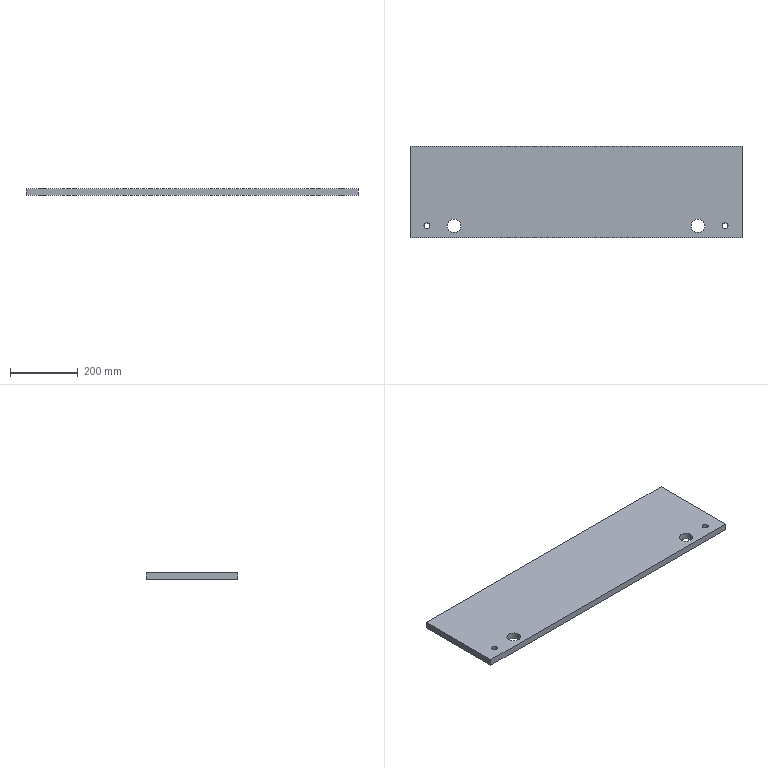Part | STEP file | Base Plate | 1 solid | 14 faces | box 980 x 270 x 20 mm | volume 5232113 mm3 | cylinder 8 | plane 6 | commonest cylinder face diameters 17.5 x4 40 x4
STEP:
#1=CARTESIAN_POINT('',(0.,0.,0.));
#2=DIRECTION('',(0.,0.,1.));
#3=DIRECTION('',(1.,0.,0.));
#4=AXIS2_PLACEMENT_3D('',#1,#2,#3);
#5=CARTESIAN_POINT('',(-340.,-100.,0.));
#6=VERTEX_POINT('',#5);
#7=CARTESIAN_POINT('',(-340.,-100.,20.));
#8=VERTEX_POINT('',#7);
#9=CARTESIAN_POINT('',(-340.,-100.,20.));
#10=DIRECTION('',(0.,0.,1.));
#11=VECTOR('',#10,1.);
#12=LINE('',#9,#11);
#13=CARTESIAN_POINT('',(-360.,-100.,20.));
#14=DIRECTION('',(0.,0.,1.));
#15=DIRECTION('',(1.,0.,0.));
#16=AXIS2_PLACEMENT_3D('',#13,#14,#15);
#17=CYLINDRICAL_SURFACE('',#16,20.);
#18=CARTESIAN_POINT('',(6.283,0.));
#19=DIRECTION('',(0.,1.));
#20=VECTOR('',#19,1.);
#21=LINE('',#18,#20);
#22=(GEOMETRIC_REPRESENTATION_CONTEXT(2)PARAMETRIC_REPRESENTATION_CONTEXT()REPRESENTATION_CONTEXT('',''));
#23=DEFINITIONAL_REPRESENTATION('',(#21),#22);
#24=PCURVE('',#17,#23);
#25=CARTESIAN_POINT('',(-360.,-100.,20.));
#26=DIRECTION('',(0.,0.,1.));
#27=DIRECTION('',(1.,0.,0.));
#28=AXIS2_PLACEMENT_3D('',#25,#26,#27);
#29=CYLINDRICAL_SURFACE('',#28,20.);
#30=CARTESIAN_POINT('',(0.,0.));
#31=DIRECTION('',(0.,1.));
#32=VECTOR('',#31,1.);
#33=LINE('',#30,#32);
#34=(GEOMETRIC_REPRESENTATION_CONTEXT(2)PARAMETRIC_REPRESENTATION_CONTEXT()REPRESENTATION_CONTEXT('',''));
#35=DEFINITIONAL_REPRESENTATION('',(#33),#34);
#36=PCURVE('',#29,#35);
#37=SURFACE_CURVE('',#12,(#24,#36),.PCURVE_S1.);
#38=EDGE_CURVE('',#6,#8,#37,.T.);
#39=ORIENTED_EDGE('',*,*,#38,.T.);
#40=CARTESIAN_POINT('',(-380.,-100.,20.));
#41=VERTEX_POINT('',#40);
#42=CARTESIAN_POINT('',(-360.,-100.,20.));
#43=DIRECTION('',(0.,0.,1.));
#44=DIRECTION('',(1.,0.,0.));
#45=AXIS2_PLACEMENT_3D('',#42,#43,#44);
#46=CIRCLE('',#45,20.);
#47=CARTESIAN_POINT('',(0.,0.));
#48=DIRECTION('',(1.,0.));
#49=VECTOR('',#48,1.);
#50=LINE('',#47,#49);
#51=(GEOMETRIC_REPRESENTATION_CONTEXT(2)PARAMETRIC_REPRESENTATION_CONTEXT()REPRESENTATION_CONTEXT('',''));
#52=DEFINITIONAL_REPRESENTATION('',(#50),#51);
#53=PCURVE('',#17,#52);
#54=CARTESIAN_POINT('',(0.,0.,20.));
#55=DIRECTION('',(0.,0.,1.));
#56=DIRECTION('',(1.,0.,0.));
#57=AXIS2_PLACEMENT_3D('',#54,#55,#56);
#58=PLANE('',#57);
#59=CARTESIAN_POINT('',(-360.,-100.));
#60=DIRECTION('',(1.,0.));
#61=AXIS2_PLACEMENT_2D('',#59,#60);
#62=CIRCLE('',#61,20.);
#63=(GEOMETRIC_REPRESENTATION_CONTEXT(2)PARAMETRIC_REPRESENTATION_CONTEXT()REPRESENTATION_CONTEXT('',''));
#64=DEFINITIONAL_REPRESENTATION('',(#62),#63);
#65=PCURVE('',#58,#64);
#66=SURFACE_CURVE('',#46,(#53,#65),.PCURVE_S1.);
#67=EDGE_CURVE('',#41,#8,#66,.T.);
#68=ORIENTED_EDGE('',*,*,#67,.F.);
#69=CARTESIAN_POINT('',(-380.,-100.,0.));
#70=VERTEX_POINT('',#69);
#71=CARTESIAN_POINT('',(-380.,-100.,20.));
#72=DIRECTION('',(0.,0.,1.));
#73=VECTOR('',#72,1.);
#74=LINE('',#71,#73);
#75=CARTESIAN_POINT('',(3.142,0.));
#76=DIRECTION('',(0.,1.));
#77=VECTOR('',#76,1.);
#78=LINE('',#75,#77);
#79=(GEOMETRIC_REPRESENTATION_CONTEXT(2)PARAMETRIC_REPRESENTATION_CONTEXT()REPRESENTATION_CONTEXT('',''));
#80=DEFINITIONAL_REPRESENTATION('',(#78),#79);
#81=PCURVE('',#17,#80);
#82=CARTESIAN_POINT('',(3.142,0.));
#83=DIRECTION('',(0.,1.));
#84=VECTOR('',#83,1.);
#85=LINE('',#82,#84);
#86=(GEOMETRIC_REPRESENTATION_CONTEXT(2)PARAMETRIC_REPRESENTATION_CONTEXT()REPRESENTATION_CONTEXT('',''));
#87=DEFINITIONAL_REPRESENTATION('',(#85),#86);
#88=PCURVE('',#29,#87);
#89=SURFACE_CURVE('',#74,(#81,#88),.PCURVE_S1.);
#90=EDGE_CURVE('',#70,#41,#89,.T.);
#91=ORIENTED_EDGE('',*,*,#90,.F.);
#92=CARTESIAN_POINT('',(-360.,-100.,0.));
#93=DIRECTION('',(0.,0.,1.));
#94=DIRECTION('',(1.,0.,0.));
#95=AXIS2_PLACEMENT_3D('',#92,#93,#94);
#96=CIRCLE('',#95,20.);
#97=CARTESIAN_POINT('',(0.,-20.));
#98=DIRECTION('',(1.,0.));
#99=VECTOR('',#98,1.);
#100=LINE('',#97,#99);
#101=(GEOMETRIC_REPRESENTATION_CONTEXT(2)PARAMETRIC_REPRESENTATION_CONTEXT()REPRESENTATION_CONTEXT('',''));
#102=DEFINITIONAL_REPRESENTATION('',(#100),#101);
#103=PCURVE('',#17,#102);
#104=CARTESIAN_POINT('',(0.,0.,0.));
#105=DIRECTION('',(0.,0.,1.));
#106=DIRECTION('',(1.,0.,0.));
#107=AXIS2_PLACEMENT_3D('',#104,#105,#106);
#108=PLANE('',#107);
#109=CARTESIAN_POINT('',(-360.,-100.));
#110=DIRECTION('',(1.,0.));
#111=AXIS2_PLACEMENT_2D('',#109,#110);
#112=CIRCLE('',#111,20.);
#113=(GEOMETRIC_REPRESENTATION_CONTEXT(2)PARAMETRIC_REPRESENTATION_CONTEXT()REPRESENTATION_CONTEXT('',''));
#114=DEFINITIONAL_REPRESENTATION('',(#112),#113);
#115=PCURVE('',#108,#114);
#116=SURFACE_CURVE('',#96,(#103,#115),.PCURVE_S1.);
#117=EDGE_CURVE('',#70,#6,#116,.T.);
#118=ORIENTED_EDGE('',*,*,#117,.T.);
#119=EDGE_LOOP('',(#39,#68,#91,#118));
#120=FACE_BOUND('',#119,.F.);
#121=ADVANCED_FACE('',(#120),#17,.F.);
#122=CARTESIAN_POINT('',(380.,-100.,0.));
#123=VERTEX_POINT('',#122);
#124=CARTESIAN_POINT('',(380.,-100.,20.));
#125=VERTEX_POINT('',#124);
#126=CARTESIAN_POINT('',(380.,-100.,20.));
#127=DIRECTION('',(0.,0.,1.));
#128=VECTOR('',#127,1.);
#129=LINE('',#126,#128);
#130=CARTESIAN_POINT('',(360.,-100.,20.));
#131=DIRECTION('',(0.,0.,1.));
#132=DIRECTION('',(1.,0.,0.));
#133=AXIS2_PLACEMENT_3D('',#130,#131,#132);
#134=CYLINDRICAL_SURFACE('',#133,20.);
#135=CARTESIAN_POINT('',(6.283,0.));
#136=DIRECTION('',(0.,1.));
#137=VECTOR('',#136,1.);
#138=LINE('',#135,#137);
#139=(GEOMETRIC_REPRESENTATION_CONTEXT(2)PARAMETRIC_REPRESENTATION_CONTEXT()REPRESENTATION_CONTEXT('',''));
#140=DEFINITIONAL_REPRESENTATION('',(#138),#139);
#141=PCURVE('',#134,#140);
#142=CARTESIAN_POINT('',(360.,-100.,20.));
#143=DIRECTION('',(0.,0.,1.));
#144=DIRECTION('',(1.,0.,0.));
#145=AXIS2_PLACEMENT_3D('',#142,#143,#144);
#146=CYLINDRICAL_SURFACE('',#145,20.);
#147=CARTESIAN_POINT('',(0.,0.));
#148=DIRECTION('',(0.,1.));
#149=VECTOR('',#148,1.);
#150=LINE('',#147,#149);
#151=(GEOMETRIC_REPRESENTATION_CONTEXT(2)PARAMETRIC_REPRESENTATION_CONTEXT()REPRESENTATION_CONTEXT('',''));
#152=DEFINITIONAL_REPRESENTATION('',(#150),#151);
#153=PCURVE('',#146,#152);
#154=SURFACE_CURVE('',#129,(#141,#153),.PCURVE_S1.);
#155=EDGE_CURVE('',#123,#125,#154,.T.);
#156=ORIENTED_EDGE('',*,*,#155,.T.);
#157=CARTESIAN_POINT('',(340.,-100.,20.));
#158=VERTEX_POINT('',#157);
#159=CARTESIAN_POINT('',(360.,-100.,20.));
#160=DIRECTION('',(0.,0.,1.));
#161=DIRECTION('',(1.,0.,0.));
#162=AXIS2_PLACEMENT_3D('',#159,#160,#161);
#163=CIRCLE('',#162,20.);
#164=CARTESIAN_POINT('',(0.,0.));
#165=DIRECTION('',(1.,0.));
#166=VECTOR('',#165,1.);
#167=LINE('',#164,#166);
#168=(GEOMETRIC_REPRESENTATION_CONTEXT(2)PARAMETRIC_REPRESENTATION_CONTEXT()REPRESENTATION_CONTEXT('',''));
#169=DEFINITIONAL_REPRESENTATION('',(#167),#168);
#170=PCURVE('',#134,#169);
#171=CARTESIAN_POINT('',(360.,-100.));
#172=DIRECTION('',(1.,0.));
#173=AXIS2_PLACEMENT_2D('',#171,#172);
#174=CIRCLE('',#173,20.);
#175=(GEOMETRIC_REPRESENTATION_CONTEXT(2)PARAMETRIC_REPRESENTATION_CONTEXT()REPRESENTATION_CONTEXT('',''));
#176=DEFINITIONAL_REPRESENTATION('',(#174),#175);
#177=PCURVE('',#58,#176);
#178=SURFACE_CURVE('',#163,(#170,#177),.PCURVE_S1.);
#179=EDGE_CURVE('',#158,#125,#178,.T.);
#180=ORIENTED_EDGE('',*,*,#179,.F.);
#181=CARTESIAN_POINT('',(340.,-100.,0.));
#182=VERTEX_POINT('',#181);
#183=CARTESIAN_POINT('',(340.,-100.,20.));
#184=DIRECTION('',(0.,0.,1.));
#185=VECTOR('',#184,1.);
#186=LINE('',#183,#185);
#187=CARTESIAN_POINT('',(3.142,0.));
#188=DIRECTION('',(0.,1.));
#189=VECTOR('',#188,1.);
#190=LINE('',#187,#189);
#191=(GEOMETRIC_REPRESENTATION_CONTEXT(2)PARAMETRIC_REPRESENTATION_CONTEXT()REPRESENTATION_CONTEXT('',''));
#192=DEFINITIONAL_REPRESENTATION('',(#190),#191);
#193=PCURVE('',#134,#192);
#194=CARTESIAN_POINT('',(3.142,0.));
#195=DIRECTION('',(0.,1.));
#196=VECTOR('',#195,1.);
#197=LINE('',#194,#196);
#198=(GEOMETRIC_REPRESENTATION_CONTEXT(2)PARAMETRIC_REPRESENTATION_CONTEXT()REPRESENTATION_CONTEXT('',''));
#199=DEFINITIONAL_REPRESENTATION('',(#197),#198);
#200=PCURVE('',#146,#199);
#201=SURFACE_CURVE('',#186,(#193,#200),.PCURVE_S1.);
#202=EDGE_CURVE('',#182,#158,#201,.T.);
#203=ORIENTED_EDGE('',*,*,#202,.F.);
#204=CARTESIAN_POINT('',(360.,-100.,0.));
#205=DIRECTION('',(0.,0.,1.));
#206=DIRECTION('',(1.,0.,0.));
#207=AXIS2_PLACEMENT_3D('',#204,#205,#206);
#208=CIRCLE('',#207,20.);
#209=CARTESIAN_POINT('',(0.,-20.));
#210=DIRECTION('',(1.,0.));
#211=VECTOR('',#210,1.);
#212=LINE('',#209,#211);
#213=(GEOMETRIC_REPRESENTATION_CONTEXT(2)PARAMETRIC_REPRESENTATION_CONTEXT()REPRESENTATION_CONTEXT('',''));
#214=DEFINITIONAL_REPRESENTATION('',(#212),#213);
#215=PCURVE('',#134,#214);
#216=CARTESIAN_POINT('',(360.,-100.));
#217=DIRECTION('',(1.,0.));
#218=AXIS2_PLACEMENT_2D('',#216,#217);
#219=CIRCLE('',#218,20.);
#220=(GEOMETRIC_REPRESENTATION_CONTEXT(2)PARAMETRIC_REPRESENTATION_CONTEXT()REPRESENTATION_CONTEXT('',''));
#221=DEFINITIONAL_REPRESENTATION('',(#219),#220);
#222=PCURVE('',#108,#221);
#223=SURFACE_CURVE('',#208,(#215,#222),.PCURVE_S1.);
#224=EDGE_CURVE('',#182,#123,#223,.T.);
#225=ORIENTED_EDGE('',*,*,#224,.T.);
#226=EDGE_LOOP('',(#156,#180,#203,#225));
#227=FACE_BOUND('',#226,.F.);
#228=ADVANCED_FACE('',(#227),#134,.F.);
#229=CARTESIAN_POINT('',(-431.25,-100.,0.));
#230=VERTEX_POINT('',#229);
#231=CARTESIAN_POINT('',(-431.25,-100.,20.));
#232=VERTEX_POINT('',#231);
#233=CARTESIAN_POINT('',(-431.25,-100.,20.));
#234=DIRECTION('',(0.,0.,1.));
#235=VECTOR('',#234,1.);
#236=LINE('',#233,#235);
#237=CARTESIAN_POINT('',(-440.,-100.,20.));
#238=DIRECTION('',(0.,0.,1.));
#239=DIRECTION('',(1.,0.,0.));
#240=AXIS2_PLACEMENT_3D('',#237,#238,#239);
#241=CYLINDRICAL_SURFACE('',#240,8.75);
#242=CARTESIAN_POINT('',(6.283,0.));
#243=DIRECTION('',(0.,1.));
#244=VECTOR('',#243,1.);
#245=LINE('',#242,#244);
#246=(GEOMETRIC_REPRESENTATION_CONTEXT(2)PARAMETRIC_REPRESENTATION_CONTEXT()REPRESENTATION_CONTEXT('',''));
#247=DEFINITIONAL_REPRESENTATION('',(#245),#246);
#248=PCURVE('',#241,#247);
#249=CARTESIAN_POINT('',(-440.,-100.,20.));
#250=DIRECTION('',(0.,0.,1.));
#251=DIRECTION('',(1.,0.,0.));
#252=AXIS2_PLACEMENT_3D('',#249,#250,#251);
#253=CYLINDRICAL_SURFACE('',#252,8.75);
#254=CARTESIAN_POINT('',(0.,0.));
#255=DIRECTION('',(0.,1.));
#256=VECTOR('',#255,1.);
#257=LINE('',#254,#256);
#258=(GEOMETRIC_REPRESENTATION_CONTEXT(2)PARAMETRIC_REPRESENTATION_CONTEXT()REPRESENTATION_CONTEXT('',''));
#259=DEFINITIONAL_REPRESENTATION('',(#257),#258);
#260=PCURVE('',#253,#259);
#261=SURFACE_CURVE('',#236,(#248,#260),.PCURVE_S1.);
#262=EDGE_CURVE('',#230,#232,#261,.T.);
#263=ORIENTED_EDGE('',*,*,#262,.T.);
#264=CARTESIAN_POINT('',(-448.75,-100.,20.));
#265=VERTEX_POINT('',#264);
#266=CARTESIAN_POINT('',(-440.,-100.,20.));
#267=DIRECTION('',(0.,0.,1.));
#268=DIRECTION('',(1.,0.,0.));
#269=AXIS2_PLACEMENT_3D('',#266,#267,#268);
#270=CIRCLE('',#269,8.75);
#271=CARTESIAN_POINT('',(0.,0.));
#272=DIRECTION('',(1.,0.));
#273=VECTOR('',#272,1.);
#274=LINE('',#271,#273);
#275=(GEOMETRIC_REPRESENTATION_CONTEXT(2)PARAMETRIC_REPRESENTATION_CONTEXT()REPRESENTATION_CONTEXT('',''));
#276=DEFINITIONAL_REPRESENTATION('',(#274),#275);
#277=PCURVE('',#241,#276);
#278=CARTESIAN_POINT('',(-440.,-100.));
#279=DIRECTION('',(1.,0.));
#280=AXIS2_PLACEMENT_2D('',#278,#279);
#281=CIRCLE('',#280,8.75);
#282=(GEOMETRIC_REPRESENTATION_CONTEXT(2)PARAMETRIC_REPRESENTATION_CONTEXT()REPRESENTATION_CONTEXT('',''));
#283=DEFINITIONAL_REPRESENTATION('',(#281),#282);
#284=PCURVE('',#58,#283);
#285=SURFACE_CURVE('',#270,(#277,#284),.PCURVE_S1.);
#286=EDGE_CURVE('',#265,#232,#285,.T.);
#287=ORIENTED_EDGE('',*,*,#286,.F.);
#288=CARTESIAN_POINT('',(-448.75,-100.,0.));
#289=VERTEX_POINT('',#288);
#290=CARTESIAN_POINT('',(-448.75,-100.,20.));
#291=DIRECTION('',(0.,0.,1.));
#292=VECTOR('',#291,1.);
#293=LINE('',#290,#292);
#294=CARTESIAN_POINT('',(3.142,0.));
#295=DIRECTION('',(0.,1.));
#296=VECTOR('',#295,1.);
#297=LINE('',#294,#296);
#298=(GEOMETRIC_REPRESENTATION_CONTEXT(2)PARAMETRIC_REPRESENTATION_CONTEXT()REPRESENTATION_CONTEXT('',''));
#299=DEFINITIONAL_REPRESENTATION('',(#297),#298);
#300=PCURVE('',#241,#299);
#301=CARTESIAN_POINT('',(3.142,0.));
#302=DIRECTION('',(0.,1.));
#303=VECTOR('',#302,1.);
#304=LINE('',#301,#303);
#305=(GEOMETRIC_REPRESENTATION_CONTEXT(2)PARAMETRIC_REPRESENTATION_CONTEXT()REPRESENTATION_CONTEXT('',''));
#306=DEFINITIONAL_REPRESENTATION('',(#304),#305);
#307=PCURVE('',#253,#306);
#308=SURFACE_CURVE('',#293,(#300,#307),.PCURVE_S1.);
#309=EDGE_CURVE('',#289,#265,#308,.T.);
#310=ORIENTED_EDGE('',*,*,#309,.F.);
#311=CARTESIAN_POINT('',(-440.,-100.,0.));
#312=DIRECTION('',(0.,0.,1.));
#313=DIRECTION('',(1.,0.,0.));
#314=AXIS2_PLACEMENT_3D('',#311,#312,#313);
#315=CIRCLE('',#314,8.75);
#316=CARTESIAN_POINT('',(0.,-20.));
#317=DIRECTION('',(1.,0.));
#318=VECTOR('',#317,1.);
#319=LINE('',#316,#318);
#320=(GEOMETRIC_REPRESENTATION_CONTEXT(2)PARAMETRIC_REPRESENTATION_CONTEXT()REPRESENTATION_CONTEXT('',''));
#321=DEFINITIONAL_REPRESENTATION('',(#319),#320);
#322=PCURVE('',#241,#321);
#323=CARTESIAN_POINT('',(-440.,-100.));
#324=DIRECTION('',(1.,0.));
#325=AXIS2_PLACEMENT_2D('',#323,#324);
#326=CIRCLE('',#325,8.75);
#327=(GEOMETRIC_REPRESENTATION_CONTEXT(2)PARAMETRIC_REPRESENTATION_CONTEXT()REPRESENTATION_CONTEXT('',''));
#328=DEFINITIONAL_REPRESENTATION('',(#326),#327);
#329=PCURVE('',#108,#328);
#330=SURFACE_CURVE('',#315,(#322,#329),.PCURVE_S1.);
#331=EDGE_CURVE('',#289,#230,#330,.T.);
#332=ORIENTED_EDGE('',*,*,#331,.T.);
#333=EDGE_LOOP('',(#263,#287,#310,#332));
#334=FACE_BOUND('',#333,.F.);
#335=ADVANCED_FACE('',(#334),#241,.F.);
#336=CARTESIAN_POINT('',(448.75,-100.,0.));
#337=VERTEX_POINT('',#336);
#338=CARTESIAN_POINT('',(448.75,-100.,20.));
#339=VERTEX_POINT('',#338);
#340=CARTESIAN_POINT('',(448.75,-100.,20.));
#341=DIRECTION('',(0.,0.,1.));
#342=VECTOR('',#341,1.);
#343=LINE('',#340,#342);
#344=CARTESIAN_POINT('',(440.,-100.,20.));
#345=DIRECTION('',(0.,0.,1.));
#346=DIRECTION('',(1.,0.,0.));
#347=AXIS2_PLACEMENT_3D('',#344,#345,#346);
#348=CYLINDRICAL_SURFACE('',#347,8.75);
#349=CARTESIAN_POINT('',(6.283,0.));
#350=DIRECTION('',(0.,1.));
#351=VECTOR('',#350,1.);
#352=LINE('',#349,#351);
#353=(GEOMETRIC_REPRESENTATION_CONTEXT(2)PARAMETRIC_REPRESENTATION_CONTEXT()REPRESENTATION_CONTEXT('',''));
#354=DEFINITIONAL_REPRESENTATION('',(#352),#353);
#355=PCURVE('',#348,#354);
#356=CARTESIAN_POINT('',(440.,-100.,20.));
#357=DIRECTION('',(0.,0.,1.));
#358=DIRECTION('',(1.,0.,0.));
#359=AXIS2_PLACEMENT_3D('',#356,#357,#358);
#360=CYLINDRICAL_SURFACE('',#359,8.75);
#361=CARTESIAN_POINT('',(0.,0.));
#362=DIRECTION('',(0.,1.));
#363=VECTOR('',#362,1.);
#364=LINE('',#361,#363);
#365=(GEOMETRIC_REPRESENTATION_CONTEXT(2)PARAMETRIC_REPRESENTATION_CONTEXT()REPRESENTATION_CONTEXT('',''));
#366=DEFINITIONAL_REPRESENTATION('',(#364),#365);
#367=PCURVE('',#360,#366);
#368=SURFACE_CURVE('',#343,(#355,#367),.PCURVE_S1.);
#369=EDGE_CURVE('',#337,#339,#368,.T.);
#370=ORIENTED_EDGE('',*,*,#369,.T.);
#371=CARTESIAN_POINT('',(431.25,-100.,20.));
#372=VERTEX_POINT('',#371);
#373=CARTESIAN_POINT('',(440.,-100.,20.));
#374=DIRECTION('',(0.,0.,1.));
#375=DIRECTION('',(1.,0.,0.));
#376=AXIS2_PLACEMENT_3D('',#373,#374,#375);
#377=CIRCLE('',#376,8.75);
#378=CARTESIAN_POINT('',(0.,0.));
#379=DIRECTION('',(1.,0.));
#380=VECTOR('',#379,1.);
#381=LINE('',#378,#380);
#382=(GEOMETRIC_REPRESENTATION_CONTEXT(2)PARAMETRIC_REPRESENTATION_CONTEXT()REPRESENTATION_CONTEXT('',''));
#383=DEFINITIONAL_REPRESENTATION('',(#381),#382);
#384=PCURVE('',#348,#383);
#385=CARTESIAN_POINT('',(440.,-100.));
#386=DIRECTION('',(1.,0.));
#387=AXIS2_PLACEMENT_2D('',#385,#386);
#388=CIRCLE('',#387,8.75);
#389=(GEOMETRIC_REPRESENTATION_CONTEXT(2)PARAMETRIC_REPRESENTATION_CONTEXT()REPRESENTATION_CONTEXT('',''));
#390=DEFINITIONAL_REPRESENTATION('',(#388),#389);
#391=PCURVE('',#58,#390);
#392=SURFACE_CURVE('',#377,(#384,#391),.PCURVE_S1.);
#393=EDGE_CURVE('',#372,#339,#392,.T.);
#394=ORIENTED_EDGE('',*,*,#393,.F.);
#395=CARTESIAN_POINT('',(431.25,-100.,0.));
#396=VERTEX_POINT('',#395);
#397=CARTESIAN_POINT('',(431.25,-100.,20.));
#398=DIRECTION('',(0.,0.,1.));
#399=VECTOR('',#398,1.);
#400=LINE('',#397,#399);
#401=CARTESIAN_POINT('',(3.142,0.));
#402=DIRECTION('',(0.,1.));
#403=VECTOR('',#402,1.);
#404=LINE('',#401,#403);
#405=(GEOMETRIC_REPRESENTATION_CONTEXT(2)PARAMETRIC_REPRESENTATION_CONTEXT()REPRESENTATION_CONTEXT('',''));
#406=DEFINITIONAL_REPRESENTATION('',(#404),#405);
#407=PCURVE('',#348,#406);
#408=CARTESIAN_POINT('',(3.142,0.));
#409=DIRECTION('',(0.,1.));
#410=VECTOR('',#409,1.);
#411=LINE('',#408,#410);
#412=(GEOMETRIC_REPRESENTATION_CONTEXT(2)PARAMETRIC_REPRESENTATION_CONTEXT()REPRESENTATION_CONTEXT('',''));
#413=DEFINITIONAL_REPRESENTATION('',(#411),#412);
#414=PCURVE('',#360,#413);
#415=SURFACE_CURVE('',#400,(#407,#414),.PCURVE_S1.);
#416=EDGE_CURVE('',#396,#372,#415,.T.);
#417=ORIENTED_EDGE('',*,*,#416,.F.);
#418=CARTESIAN_POINT('',(440.,-100.,0.));
#419=DIRECTION('',(0.,0.,1.));
#420=DIRECTION('',(1.,0.,0.));
#421=AXIS2_PLACEMENT_3D('',#418,#419,#420);
#422=CIRCLE('',#421,8.75);
#423=CARTESIAN_POINT('',(0.,-20.));
#424=DIRECTION('',(1.,0.));
#425=VECTOR('',#424,1.);
#426=LINE('',#423,#425);
#427=(GEOMETRIC_REPRESENTATION_CONTEXT(2)PARAMETRIC_REPRESENTATION_CONTEXT()REPRESENTATION_CONTEXT('',''));
#428=DEFINITIONAL_REPRESENTATION('',(#426),#427);
#429=PCURVE('',#348,#428);
#430=CARTESIAN_POINT('',(440.,-100.));
#431=DIRECTION('',(1.,0.));
#432=AXIS2_PLACEMENT_2D('',#430,#431);
#433=CIRCLE('',#432,8.75);
#434=(GEOMETRIC_REPRESENTATION_CONTEXT(2)PARAMETRIC_REPRESENTATION_CONTEXT()REPRESENTATION_CONTEXT('',''));
#435=DEFINITIONAL_REPRESENTATION('',(#433),#434);
#436=PCURVE('',#108,#435);
#437=SURFACE_CURVE('',#422,(#429,#436),.PCURVE_S1.);
#438=EDGE_CURVE('',#396,#337,#437,.T.);
#439=ORIENTED_EDGE('',*,*,#438,.T.);
#440=EDGE_LOOP('',(#370,#394,#417,#439));
#441=FACE_BOUND('',#440,.F.);
#442=ADVANCED_FACE('',(#441),#348,.F.);
#443=CARTESIAN_POINT('',(490.,-135.,0.));
#444=VERTEX_POINT('',#443);
#445=CARTESIAN_POINT('',(490.,135.,0.));
#446=VERTEX_POINT('',#445);
#447=CARTESIAN_POINT('',(490.,135.,0.));
#448=DIRECTION('',(0.,1.,0.));
#449=VECTOR('',#448,1.);
#450=LINE('',#447,#449);
#451=CARTESIAN_POINT('',(490.,135.,20.));
#452=DIRECTION('',(-1.,0.,0.));
#453=DIRECTION('',(0.,-1.,0.));
#454=AXIS2_PLACEMENT_3D('',#451,#452,#453);
#455=PLANE('',#454);
#456=CARTESIAN_POINT('',(0.,-20.));
#457=DIRECTION('',(-1.,0.));
#458=VECTOR('',#457,1.);
#459=LINE('',#456,#458);
#460=(GEOMETRIC_REPRESENTATION_CONTEXT(2)PARAMETRIC_REPRESENTATION_CONTEXT()REPRESENTATION_CONTEXT('',''));
#461=DEFINITIONAL_REPRESENTATION('',(#459),#460);
#462=PCURVE('',#455,#461);
#463=CARTESIAN_POINT('',(490.,135.));
#464=DIRECTION('',(0.,1.));
#465=VECTOR('',#464,1.);
#466=LINE('',#463,#465);
#467=(GEOMETRIC_REPRESENTATION_CONTEXT(2)PARAMETRIC_REPRESENTATION_CONTEXT()REPRESENTATION_CONTEXT('',''));
#468=DEFINITIONAL_REPRESENTATION('',(#466),#467);
#469=PCURVE('',#108,#468);
#470=SURFACE_CURVE('',#450,(#462,#469),.PCURVE_S1.);
#471=EDGE_CURVE('',#444,#446,#470,.T.);
#472=ORIENTED_EDGE('',*,*,#471,.T.);
#473=CARTESIAN_POINT('',(490.,135.,20.));
#474=VERTEX_POINT('',#473);
#475=CARTESIAN_POINT('',(490.,135.,20.));
#476=DIRECTION('',(0.,0.,-1.));
#477=VECTOR('',#476,1.);
#478=LINE('',#475,#477);
#479=CARTESIAN_POINT('',(0.,0.));
#480=DIRECTION('',(0.,-1.));
#481=VECTOR('',#480,1.);
#482=LINE('',#479,#481);
#483=(GEOMETRIC_REPRESENTATION_CONTEXT(2)PARAMETRIC_REPRESENTATION_CONTEXT()REPRESENTATION_CONTEXT('',''));
#484=DEFINITIONAL_REPRESENTATION('',(#482),#483);
#485=PCURVE('',#455,#484);
#486=CARTESIAN_POINT('',(-490.,135.,20.));
#487=DIRECTION('',(0.,-1.,0.));
#488=DIRECTION('',(0.,0.,-1.));
#489=AXIS2_PLACEMENT_3D('',#486,#487,#488);
#490=PLANE('',#489);
#491=CARTESIAN_POINT('',(0.,980.));
#492=DIRECTION('',(1.,0.));
#493=VECTOR('',#492,1.);
#494=LINE('',#491,#493);
#495=(GEOMETRIC_REPRESENTATION_CONTEXT(2)PARAMETRIC_REPRESENTATION_CONTEXT()REPRESENTATION_CONTEXT('',''));
#496=DEFINITIONAL_REPRESENTATION('',(#494),#495);
#497=PCURVE('',#490,#496);
#498=SURFACE_CURVE('',#478,(#485,#497),.PCURVE_S1.);
#499=EDGE_CURVE('',#474,#446,#498,.T.);
#500=ORIENTED_EDGE('',*,*,#499,.F.);
#501=CARTESIAN_POINT('',(490.,-135.,20.));
#502=VERTEX_POINT('',#501);
#503=CARTESIAN_POINT('',(490.,135.,20.));
#504=DIRECTION('',(0.,1.,0.));
#505=VECTOR('',#504,1.);
#506=LINE('',#503,#505);
#507=CARTESIAN_POINT('',(0.,0.));
#508=DIRECTION('',(-1.,0.));
#509=VECTOR('',#508,1.);
#510=LINE('',#507,#509);
#511=(GEOMETRIC_REPRESENTATION_CONTEXT(2)PARAMETRIC_REPRESENTATION_CONTEXT()REPRESENTATION_CONTEXT('',''));
#512=DEFINITIONAL_REPRESENTATION('',(#510),#511);
#513=PCURVE('',#455,#512);
#514=CARTESIAN_POINT('',(490.,135.));
#515=DIRECTION('',(0.,1.));
#516=VECTOR('',#515,1.);
#517=LINE('',#514,#516);
#518=(GEOMETRIC_REPRESENTATION_CONTEXT(2)PARAMETRIC_REPRESENTATION_CONTEXT()REPRESENTATION_CONTEXT('',''));
#519=DEFINITIONAL_REPRESENTATION('',(#517),#518);
#520=PCURVE('',#58,#519);
#521=SURFACE_CURVE('',#506,(#513,#520),.PCURVE_S1.);
#522=EDGE_CURVE('',#502,#474,#521,.T.);
#523=ORIENTED_EDGE('',*,*,#522,.F.);
#524=CARTESIAN_POINT('',(490.,-135.,20.));
#525=DIRECTION('',(0.,0.,-1.));
#526=VECTOR('',#525,1.);
#527=LINE('',#524,#526);
#528=CARTESIAN_POINT('',(270.,0.));
#529=DIRECTION('',(0.,-1.));
#530=VECTOR('',#529,1.);
#531=LINE('',#528,#530);
#532=(GEOMETRIC_REPRESENTATION_CONTEXT(2)PARAMETRIC_REPRESENTATION_CONTEXT()REPRESENTATION_CONTEXT('',''));
#533=DEFINITIONAL_REPRESENTATION('',(#531),#532);
#534=PCURVE('',#455,#533);
#535=CARTESIAN_POINT('',(-490.,-135.,20.));
#536=DIRECTION('',(0.,1.,0.));
#537=DIRECTION('',(0.,0.,1.));
#538=AXIS2_PLACEMENT_3D('',#535,#536,#537);
#539=PLANE('',#538);
#540=CARTESIAN_POINT('',(0.,980.));
#541=DIRECTION('',(-1.,0.));
#542=VECTOR('',#541,1.);
#543=LINE('',#540,#542);
#544=(GEOMETRIC_REPRESENTATION_CONTEXT(2)PARAMETRIC_REPRESENTATION_CONTEXT()REPRESENTATION_CONTEXT('',''));
#545=DEFINITIONAL_REPRESENTATION('',(#543),#544);
#546=PCURVE('',#539,#545);
#547=SURFACE_CURVE('',#527,(#534,#546),.PCURVE_S1.);
#548=EDGE_CURVE('',#502,#444,#547,.T.);
#549=ORIENTED_EDGE('',*,*,#548,.T.);
#550=EDGE_LOOP('',(#472,#500,#523,#549));
#551=FACE_BOUND('',#550,.T.);
#552=ADVANCED_FACE('',(#551),#455,.F.);
#553=CARTESIAN_POINT('',(-490.,135.,0.));
#554=VERTEX_POINT('',#553);
#555=CARTESIAN_POINT('',(-490.,135.,0.));
#556=DIRECTION('',(-1.,0.,0.));
#557=VECTOR('',#556,1.);
#558=LINE('',#555,#557);
#559=CARTESIAN_POINT('',(20.,0.));
#560=DIRECTION('',(0.,-1.));
#561=VECTOR('',#560,1.);
#562=LINE('',#559,#561);
#563=(GEOMETRIC_REPRESENTATION_CONTEXT(2)PARAMETRIC_REPRESENTATION_CONTEXT()REPRESENTATION_CONTEXT('',''));
#564=DEFINITIONAL_REPRESENTATION('',(#562),#563);
#565=PCURVE('',#490,#564);
#566=CARTESIAN_POINT('',(-490.,135.));
#567=DIRECTION('',(-1.,0.));
#568=VECTOR('',#567,1.);
#569=LINE('',#566,#568);
#570=(GEOMETRIC_REPRESENTATION_CONTEXT(2)PARAMETRIC_REPRESENTATION_CONTEXT()REPRESENTATION_CONTEXT('',''));
#571=DEFINITIONAL_REPRESENTATION('',(#569),#570);
#572=PCURVE('',#108,#571);
#573=SURFACE_CURVE('',#558,(#565,#572),.PCURVE_S1.);
#574=EDGE_CURVE('',#446,#554,#573,.T.);
#575=ORIENTED_EDGE('',*,*,#574,.T.);
#576=CARTESIAN_POINT('',(-490.,135.,20.));
#577=VERTEX_POINT('',#576);
#578=CARTESIAN_POINT('',(-490.,135.,20.));
#579=DIRECTION('',(0.,0.,-1.));
#580=VECTOR('',#579,1.);
#581=LINE('',#578,#580);
#582=CARTESIAN_POINT('',(0.,0.));
#583=DIRECTION('',(1.,0.));
#584=VECTOR('',#583,1.);
#585=LINE('',#582,#584);
#586=(GEOMETRIC_REPRESENTATION_CONTEXT(2)PARAMETRIC_REPRESENTATION_CONTEXT()REPRESENTATION_CONTEXT('',''));
#587=DEFINITIONAL_REPRESENTATION('',(#585),#586);
#588=PCURVE('',#490,#587);
#589=CARTESIAN_POINT('',(-490.,135.,20.));
#590=DIRECTION('',(1.,0.,0.));
#591=DIRECTION('',(0.,1.,0.));
#592=AXIS2_PLACEMENT_3D('',#589,#590,#591);
#593=PLANE('',#592);
#594=CARTESIAN_POINT('',(0.,0.));
#595=DIRECTION('',(0.,-1.));
#596=VECTOR('',#595,1.);
#597=LINE('',#594,#596);
#598=(GEOMETRIC_REPRESENTATION_CONTEXT(2)PARAMETRIC_REPRESENTATION_CONTEXT()REPRESENTATION_CONTEXT('',''));
#599=DEFINITIONAL_REPRESENTATION('',(#597),#598);
#600=PCURVE('',#593,#599);
#601=SURFACE_CURVE('',#581,(#588,#600),.PCURVE_S1.);
#602=EDGE_CURVE('',#577,#554,#601,.T.);
#603=ORIENTED_EDGE('',*,*,#602,.F.);
#604=CARTESIAN_POINT('',(-490.,135.,20.));
#605=DIRECTION('',(-1.,0.,0.));
#606=VECTOR('',#605,1.);
#607=LINE('',#604,#606);
#608=CARTESIAN_POINT('',(0.,0.));
#609=DIRECTION('',(0.,-1.));
#610=VECTOR('',#609,1.);
#611=LINE('',#608,#610);
#612=(GEOMETRIC_REPRESENTATION_CONTEXT(2)PARAMETRIC_REPRESENTATION_CONTEXT()REPRESENTATION_CONTEXT('',''));
#613=DEFINITIONAL_REPRESENTATION('',(#611),#612);
#614=PCURVE('',#490,#613);
#615=CARTESIAN_POINT('',(-490.,135.));
#616=DIRECTION('',(-1.,0.));
#617=VECTOR('',#616,1.);
#618=LINE('',#615,#617);
#619=(GEOMETRIC_REPRESENTATION_CONTEXT(2)PARAMETRIC_REPRESENTATION_CONTEXT()REPRESENTATION_CONTEXT('',''));
#620=DEFINITIONAL_REPRESENTATION('',(#618),#619);
#621=PCURVE('',#58,#620);
#622=SURFACE_CURVE('',#607,(#614,#621),.PCURVE_S1.);
#623=EDGE_CURVE('',#474,#577,#622,.T.);
#624=ORIENTED_EDGE('',*,*,#623,.F.);
#625=ORIENTED_EDGE('',*,*,#499,.T.);
#626=EDGE_LOOP('',(#575,#603,#624,#625));
#627=FACE_BOUND('',#626,.T.);
#628=ADVANCED_FACE('',(#627),#490,.F.);
#629=CARTESIAN_POINT('',(-490.,-135.,0.));
#630=VERTEX_POINT('',#629);
#631=CARTESIAN_POINT('',(-490.,135.,0.));
#632=DIRECTION('',(0.,-1.,0.));
#633=VECTOR('',#632,1.);
#634=LINE('',#631,#633);
#635=CARTESIAN_POINT('',(0.,-20.));
#636=DIRECTION('',(-1.,0.));
#637=VECTOR('',#636,1.);
#638=LINE('',#635,#637);
#639=(GEOMETRIC_REPRESENTATION_CONTEXT(2)PARAMETRIC_REPRESENTATION_CONTEXT()REPRESENTATION_CONTEXT('',''));
#640=DEFINITIONAL_REPRESENTATION('',(#638),#639);
#641=PCURVE('',#593,#640);
#642=CARTESIAN_POINT('',(-490.,135.));
#643=DIRECTION('',(0.,-1.));
#644=VECTOR('',#643,1.);
#645=LINE('',#642,#644);
#646=(GEOMETRIC_REPRESENTATION_CONTEXT(2)PARAMETRIC_REPRESENTATION_CONTEXT()REPRESENTATION_CONTEXT('',''));
#647=DEFINITIONAL_REPRESENTATION('',(#645),#646);
#648=PCURVE('',#108,#647);
#649=SURFACE_CURVE('',#634,(#641,#648),.PCURVE_S1.);
#650=EDGE_CURVE('',#554,#630,#649,.T.);
#651=ORIENTED_EDGE('',*,*,#650,.T.);
#652=CARTESIAN_POINT('',(-490.,-135.,20.));
#653=VERTEX_POINT('',#652);
#654=CARTESIAN_POINT('',(-490.,-135.,20.));
#655=DIRECTION('',(0.,0.,-1.));
#656=VECTOR('',#655,1.);
#657=LINE('',#654,#656);
#658=CARTESIAN_POINT('',(-270.,0.));
#659=DIRECTION('',(0.,-1.));
#660=VECTOR('',#659,1.);
#661=LINE('',#658,#660);
#662=(GEOMETRIC_REPRESENTATION_CONTEXT(2)PARAMETRIC_REPRESENTATION_CONTEXT()REPRESENTATION_CONTEXT('',''));
#663=DEFINITIONAL_REPRESENTATION('',(#661),#662);
#664=PCURVE('',#593,#663);
#665=CARTESIAN_POINT('',(0.,0.));
#666=DIRECTION('',(-1.,0.));
#667=VECTOR('',#666,1.);
#668=LINE('',#665,#667);
#669=(GEOMETRIC_REPRESENTATION_CONTEXT(2)PARAMETRIC_REPRESENTATION_CONTEXT()REPRESENTATION_CONTEXT('',''));
#670=DEFINITIONAL_REPRESENTATION('',(#668),#669);
#671=PCURVE('',#539,#670);
#672=SURFACE_CURVE('',#657,(#664,#671),.PCURVE_S1.);
#673=EDGE_CURVE('',#653,#630,#672,.T.);
#674=ORIENTED_EDGE('',*,*,#673,.F.);
#675=CARTESIAN_POINT('',(-490.,135.,20.));
#676=DIRECTION('',(0.,-1.,0.));
#677=VECTOR('',#676,1.);
#678=LINE('',#675,#677);
#679=CARTESIAN_POINT('',(0.,0.));
#680=DIRECTION('',(-1.,0.));
#681=VECTOR('',#680,1.);
#682=LINE('',#679,#681);
#683=(GEOMETRIC_REPRESENTATION_CONTEXT(2)PARAMETRIC_REPRESENTATION_CONTEXT()REPRESENTATION_CONTEXT('',''));
#684=DEFINITIONAL_REPRESENTATION('',(#682),#683);
#685=PCURVE('',#593,#684);
#686=CARTESIAN_POINT('',(-490.,135.));
#687=DIRECTION('',(0.,-1.));
#688=VECTOR('',#687,1.);
#689=LINE('',#686,#688);
#690=(GEOMETRIC_REPRESENTATION_CONTEXT(2)PARAMETRIC_REPRESENTATION_CONTEXT()REPRESENTATION_CONTEXT('',''));
#691=DEFINITIONAL_REPRESENTATION('',(#689),#690);
#692=PCURVE('',#58,#691);
#693=SURFACE_CURVE('',#678,(#685,#692),.PCURVE_S1.);
#694=EDGE_CURVE('',#577,#653,#693,.T.);
#695=ORIENTED_EDGE('',*,*,#694,.F.);
#696=ORIENTED_EDGE('',*,*,#602,.T.);
#697=EDGE_LOOP('',(#651,#674,#695,#696));
#698=FACE_BOUND('',#697,.T.);
#699=ADVANCED_FACE('',(#698),#593,.F.);
#700=CARTESIAN_POINT('',(-490.,-135.,0.));
#701=DIRECTION('',(1.,0.,0.));
#702=VECTOR('',#701,1.);
#703=LINE('',#700,#702);
#704=CARTESIAN_POINT('',(-20.,0.));
#705=DIRECTION('',(0.,1.));
#706=VECTOR('',#705,1.);
#707=LINE('',#704,#706);
#708=(GEOMETRIC_REPRESENTATION_CONTEXT(2)PARAMETRIC_REPRESENTATION_CONTEXT()REPRESENTATION_CONTEXT('',''));
#709=DEFINITIONAL_REPRESENTATION('',(#707),#708);
#710=PCURVE('',#539,#709);
#711=CARTESIAN_POINT('',(-490.,-135.));
#712=DIRECTION('',(1.,0.));
#713=VECTOR('',#712,1.);
#714=LINE('',#711,#713);
#715=(GEOMETRIC_REPRESENTATION_CONTEXT(2)PARAMETRIC_REPRESENTATION_CONTEXT()REPRESENTATION_CONTEXT('',''));
#716=DEFINITIONAL_REPRESENTATION('',(#714),#715);
#717=PCURVE('',#108,#716);
#718=SURFACE_CURVE('',#703,(#710,#717),.PCURVE_S1.);
#719=EDGE_CURVE('',#630,#444,#718,.T.);
#720=ORIENTED_EDGE('',*,*,#719,.T.);
#721=ORIENTED_EDGE('',*,*,#548,.F.);
#722=CARTESIAN_POINT('',(-490.,-135.,20.));
#723=DIRECTION('',(1.,0.,0.));
#724=VECTOR('',#723,1.);
#725=LINE('',#722,#724);
#726=CARTESIAN_POINT('',(0.,0.));
#727=DIRECTION('',(0.,1.));
#728=VECTOR('',#727,1.);
#729=LINE('',#726,#728);
#730=(GEOMETRIC_REPRESENTATION_CONTEXT(2)PARAMETRIC_REPRESENTATION_CONTEXT()REPRESENTATION_CONTEXT('',''));
#731=DEFINITIONAL_REPRESENTATION('',(#729),#730);
#732=PCURVE('',#539,#731);
#733=CARTESIAN_POINT('',(-490.,-135.));
#734=DIRECTION('',(1.,0.));
#735=VECTOR('',#734,1.);
#736=LINE('',#733,#735);
#737=(GEOMETRIC_REPRESENTATION_CONTEXT(2)PARAMETRIC_REPRESENTATION_CONTEXT()REPRESENTATION_CONTEXT('',''));
#738=DEFINITIONAL_REPRESENTATION('',(#736),#737);
#739=PCURVE('',#58,#738);
#740=SURFACE_CURVE('',#725,(#732,#739),.PCURVE_S1.);
#741=EDGE_CURVE('',#653,#502,#740,.T.);
#742=ORIENTED_EDGE('',*,*,#741,.F.);
#743=ORIENTED_EDGE('',*,*,#673,.T.);
#744=EDGE_LOOP('',(#720,#721,#742,#743));
#745=FACE_BOUND('',#744,.T.);
#746=ADVANCED_FACE('',(#745),#539,.F.);
#747=CARTESIAN_POINT('',(-360.,-100.,20.));
#748=DIRECTION('',(0.,0.,1.));
#749=DIRECTION('',(1.,0.,0.));
#750=AXIS2_PLACEMENT_3D('',#747,#748,#749);
#751=CIRCLE('',#750,20.);
#752=CARTESIAN_POINT('',(-360.,-100.));
#753=DIRECTION('',(1.,0.));
#754=AXIS2_PLACEMENT_2D('',#752,#753);
#755=CIRCLE('',#754,20.);
#756=(GEOMETRIC_REPRESENTATION_CONTEXT(2)PARAMETRIC_REPRESENTATION_CONTEXT()REPRESENTATION_CONTEXT('',''));
#757=DEFINITIONAL_REPRESENTATION('',(#755),#756);
#758=PCURVE('',#58,#757);
#759=CARTESIAN_POINT('',(0.,0.));
#760=DIRECTION('',(1.,0.));
#761=VECTOR('',#760,1.);
#762=LINE('',#759,#761);
#763=(GEOMETRIC_REPRESENTATION_CONTEXT(2)PARAMETRIC_REPRESENTATION_CONTEXT()REPRESENTATION_CONTEXT('',''));
#764=DEFINITIONAL_REPRESENTATION('',(#762),#763);
#765=PCURVE('',#29,#764);
#766=SURFACE_CURVE('',#751,(#758,#765),.PCURVE_S1.);
#767=EDGE_CURVE('',#8,#41,#766,.T.);
#768=ORIENTED_EDGE('',*,*,#767,.F.);
#769=ORIENTED_EDGE('',*,*,#67,.F.);
#770=EDGE_LOOP('',(#768,#769));
#771=FACE_BOUND('',#770,.T.);
#772=CARTESIAN_POINT('',(360.,-100.,20.));
#773=DIRECTION('',(0.,0.,1.));
#774=DIRECTION('',(1.,0.,0.));
#775=AXIS2_PLACEMENT_3D('',#772,#773,#774);
#776=CIRCLE('',#775,20.);
#777=CARTESIAN_POINT('',(360.,-100.));
#778=DIRECTION('',(1.,0.));
#779=AXIS2_PLACEMENT_2D('',#777,#778);
#780=CIRCLE('',#779,20.);
#781=(GEOMETRIC_REPRESENTATION_CONTEXT(2)PARAMETRIC_REPRESENTATION_CONTEXT()REPRESENTATION_CONTEXT('',''));
#782=DEFINITIONAL_REPRESENTATION('',(#780),#781);
#783=PCURVE('',#58,#782);
#784=CARTESIAN_POINT('',(0.,0.));
#785=DIRECTION('',(1.,0.));
#786=VECTOR('',#785,1.);
#787=LINE('',#784,#786);
#788=(GEOMETRIC_REPRESENTATION_CONTEXT(2)PARAMETRIC_REPRESENTATION_CONTEXT()REPRESENTATION_CONTEXT('',''));
#789=DEFINITIONAL_REPRESENTATION('',(#787),#788);
#790=PCURVE('',#146,#789);
#791=SURFACE_CURVE('',#776,(#783,#790),.PCURVE_S1.);
#792=EDGE_CURVE('',#125,#158,#791,.T.);
#793=ORIENTED_EDGE('',*,*,#792,.F.);
#794=ORIENTED_EDGE('',*,*,#179,.F.);
#795=EDGE_LOOP('',(#793,#794));
#796=FACE_BOUND('',#795,.T.);
#797=CARTESIAN_POINT('',(-440.,-100.,20.));
#798=DIRECTION('',(0.,0.,1.));
#799=DIRECTION('',(1.,0.,0.));
#800=AXIS2_PLACEMENT_3D('',#797,#798,#799);
#801=CIRCLE('',#800,8.75);
#802=CARTESIAN_POINT('',(-440.,-100.));
#803=DIRECTION('',(1.,0.));
#804=AXIS2_PLACEMENT_2D('',#802,#803);
#805=CIRCLE('',#804,8.75);
#806=(GEOMETRIC_REPRESENTATION_CONTEXT(2)PARAMETRIC_REPRESENTATION_CONTEXT()REPRESENTATION_CONTEXT('',''));
#807=DEFINITIONAL_REPRESENTATION('',(#805),#806);
#808=PCURVE('',#58,#807);
#809=CARTESIAN_POINT('',(0.,0.));
#810=DIRECTION('',(1.,0.));
#811=VECTOR('',#810,1.);
#812=LINE('',#809,#811);
#813=(GEOMETRIC_REPRESENTATION_CONTEXT(2)PARAMETRIC_REPRESENTATION_CONTEXT()REPRESENTATION_CONTEXT('',''));
#814=DEFINITIONAL_REPRESENTATION('',(#812),#813);
#815=PCURVE('',#253,#814);
#816=SURFACE_CURVE('',#801,(#808,#815),.PCURVE_S1.);
#817=EDGE_CURVE('',#232,#265,#816,.T.);
#818=ORIENTED_EDGE('',*,*,#817,.F.);
#819=ORIENTED_EDGE('',*,*,#286,.F.);
#820=EDGE_LOOP('',(#818,#819));
#821=FACE_BOUND('',#820,.T.);
#822=CARTESIAN_POINT('',(440.,-100.,20.));
#823=DIRECTION('',(0.,0.,1.));
#824=DIRECTION('',(1.,0.,0.));
#825=AXIS2_PLACEMENT_3D('',#822,#823,#824);
#826=CIRCLE('',#825,8.75);
#827=CARTESIAN_POINT('',(440.,-100.));
#828=DIRECTION('',(1.,0.));
#829=AXIS2_PLACEMENT_2D('',#827,#828);
#830=CIRCLE('',#829,8.75);
#831=(GEOMETRIC_REPRESENTATION_CONTEXT(2)PARAMETRIC_REPRESENTATION_CONTEXT()REPRESENTATION_CONTEXT('',''));
#832=DEFINITIONAL_REPRESENTATION('',(#830),#831);
#833=PCURVE('',#58,#832);
#834=CARTESIAN_POINT('',(0.,0.));
#835=DIRECTION('',(1.,0.));
#836=VECTOR('',#835,1.);
#837=LINE('',#834,#836);
#838=(GEOMETRIC_REPRESENTATION_CONTEXT(2)PARAMETRIC_REPRESENTATION_CONTEXT()REPRESENTATION_CONTEXT('',''));
#839=DEFINITIONAL_REPRESENTATION('',(#837),#838);
#840=PCURVE('',#360,#839);
#841=SURFACE_CURVE('',#826,(#833,#840),.PCURVE_S1.);
#842=EDGE_CURVE('',#339,#372,#841,.T.);
#843=ORIENTED_EDGE('',*,*,#842,.F.);
#844=ORIENTED_EDGE('',*,*,#393,.F.);
#845=EDGE_LOOP('',(#843,#844));
#846=FACE_BOUND('',#845,.T.);
#847=ORIENTED_EDGE('',*,*,#522,.T.);
#848=ORIENTED_EDGE('',*,*,#623,.T.);
#849=ORIENTED_EDGE('',*,*,#694,.T.);
#850=ORIENTED_EDGE('',*,*,#741,.T.);
#851=EDGE_LOOP('',(#847,#848,#849,#850));
#852=FACE_BOUND('',#851,.T.);
#853=ADVANCED_FACE('',(#771,#796,#821,#846,#852),#58,.T.);
#854=CARTESIAN_POINT('',(-360.,-100.,0.));
#855=DIRECTION('',(0.,0.,1.));
#856=DIRECTION('',(1.,0.,0.));
#857=AXIS2_PLACEMENT_3D('',#854,#855,#856);
#858=CIRCLE('',#857,20.);
#859=CARTESIAN_POINT('',(-360.,-100.));
#860=DIRECTION('',(1.,0.));
#861=AXIS2_PLACEMENT_2D('',#859,#860);
#862=CIRCLE('',#861,20.);
#863=(GEOMETRIC_REPRESENTATION_CONTEXT(2)PARAMETRIC_REPRESENTATION_CONTEXT()REPRESENTATION_CONTEXT('',''));
#864=DEFINITIONAL_REPRESENTATION('',(#862),#863);
#865=PCURVE('',#108,#864);
#866=CARTESIAN_POINT('',(0.,-20.));
#867=DIRECTION('',(1.,0.));
#868=VECTOR('',#867,1.);
#869=LINE('',#866,#868);
#870=(GEOMETRIC_REPRESENTATION_CONTEXT(2)PARAMETRIC_REPRESENTATION_CONTEXT()REPRESENTATION_CONTEXT('',''));
#871=DEFINITIONAL_REPRESENTATION('',(#869),#870);
#872=PCURVE('',#29,#871);
#873=SURFACE_CURVE('',#858,(#865,#872),.PCURVE_S1.);
#874=EDGE_CURVE('',#6,#70,#873,.T.);
#875=ORIENTED_EDGE('',*,*,#874,.T.);
#876=ORIENTED_EDGE('',*,*,#117,.T.);
#877=EDGE_LOOP('',(#875,#876));
#878=FACE_BOUND('',#877,.T.);
#879=CARTESIAN_POINT('',(360.,-100.,0.));
#880=DIRECTION('',(0.,0.,1.));
#881=DIRECTION('',(1.,0.,0.));
#882=AXIS2_PLACEMENT_3D('',#879,#880,#881);
#883=CIRCLE('',#882,20.);
#884=CARTESIAN_POINT('',(360.,-100.));
#885=DIRECTION('',(1.,0.));
#886=AXIS2_PLACEMENT_2D('',#884,#885);
#887=CIRCLE('',#886,20.);
#888=(GEOMETRIC_REPRESENTATION_CONTEXT(2)PARAMETRIC_REPRESENTATION_CONTEXT()REPRESENTATION_CONTEXT('',''));
#889=DEFINITIONAL_REPRESENTATION('',(#887),#888);
#890=PCURVE('',#108,#889);
#891=CARTESIAN_POINT('',(0.,-20.));
#892=DIRECTION('',(1.,0.));
#893=VECTOR('',#892,1.);
#894=LINE('',#891,#893);
#895=(GEOMETRIC_REPRESENTATION_CONTEXT(2)PARAMETRIC_REPRESENTATION_CONTEXT()REPRESENTATION_CONTEXT('',''));
#896=DEFINITIONAL_REPRESENTATION('',(#894),#895);
#897=PCURVE('',#146,#896);
#898=SURFACE_CURVE('',#883,(#890,#897),.PCURVE_S1.);
#899=EDGE_CURVE('',#123,#182,#898,.T.);
#900=ORIENTED_EDGE('',*,*,#899,.T.);
#901=ORIENTED_EDGE('',*,*,#224,.T.);
#902=EDGE_LOOP('',(#900,#901));
#903=FACE_BOUND('',#902,.T.);
#904=CARTESIAN_POINT('',(-440.,-100.,0.));
#905=DIRECTION('',(0.,0.,1.));
#906=DIRECTION('',(1.,0.,0.));
#907=AXIS2_PLACEMENT_3D('',#904,#905,#906);
#908=CIRCLE('',#907,8.75);
#909=CARTESIAN_POINT('',(-440.,-100.));
#910=DIRECTION('',(1.,0.));
#911=AXIS2_PLACEMENT_2D('',#909,#910);
#912=CIRCLE('',#911,8.75);
#913=(GEOMETRIC_REPRESENTATION_CONTEXT(2)PARAMETRIC_REPRESENTATION_CONTEXT()REPRESENTATION_CONTEXT('',''));
#914=DEFINITIONAL_REPRESENTATION('',(#912),#913);
#915=PCURVE('',#108,#914);
#916=CARTESIAN_POINT('',(0.,-20.));
#917=DIRECTION('',(1.,0.));
#918=VECTOR('',#917,1.);
#919=LINE('',#916,#918);
#920=(GEOMETRIC_REPRESENTATION_CONTEXT(2)PARAMETRIC_REPRESENTATION_CONTEXT()REPRESENTATION_CONTEXT('',''));
#921=DEFINITIONAL_REPRESENTATION('',(#919),#920);
#922=PCURVE('',#253,#921);
#923=SURFACE_CURVE('',#908,(#915,#922),.PCURVE_S1.);
#924=EDGE_CURVE('',#230,#289,#923,.T.);
#925=ORIENTED_EDGE('',*,*,#924,.T.);
#926=ORIENTED_EDGE('',*,*,#331,.T.);
#927=EDGE_LOOP('',(#925,#926));
#928=FACE_BOUND('',#927,.T.);
#929=CARTESIAN_POINT('',(440.,-100.,0.));
#930=DIRECTION('',(0.,0.,1.));
#931=DIRECTION('',(1.,0.,0.));
#932=AXIS2_PLACEMENT_3D('',#929,#930,#931);
#933=CIRCLE('',#932,8.75);
#934=CARTESIAN_POINT('',(440.,-100.));
#935=DIRECTION('',(1.,0.));
#936=AXIS2_PLACEMENT_2D('',#934,#935);
#937=CIRCLE('',#936,8.75);
#938=(GEOMETRIC_REPRESENTATION_CONTEXT(2)PARAMETRIC_REPRESENTATION_CONTEXT()REPRESENTATION_CONTEXT('',''));
#939=DEFINITIONAL_REPRESENTATION('',(#937),#938);
#940=PCURVE('',#108,#939);
#941=CARTESIAN_POINT('',(0.,-20.));
#942=DIRECTION('',(1.,0.));
#943=VECTOR('',#942,1.);
#944=LINE('',#941,#943);
#945=(GEOMETRIC_REPRESENTATION_CONTEXT(2)PARAMETRIC_REPRESENTATION_CONTEXT()REPRESENTATION_CONTEXT('',''));
#946=DEFINITIONAL_REPRESENTATION('',(#944),#945);
#947=PCURVE('',#360,#946);
#948=SURFACE_CURVE('',#933,(#940,#947),.PCURVE_S1.);
#949=EDGE_CURVE('',#337,#396,#948,.T.);
#950=ORIENTED_EDGE('',*,*,#949,.T.);
#951=ORIENTED_EDGE('',*,*,#438,.T.);
#952=EDGE_LOOP('',(#950,#951));
#953=FACE_BOUND('',#952,.T.);
#954=ORIENTED_EDGE('',*,*,#471,.F.);
#955=ORIENTED_EDGE('',*,*,#719,.F.);
#956=ORIENTED_EDGE('',*,*,#650,.F.);
#957=ORIENTED_EDGE('',*,*,#574,.F.);
#958=EDGE_LOOP('',(#954,#955,#956,#957));
#959=FACE_BOUND('',#958,.T.);
#960=ADVANCED_FACE('',(#878,#903,#928,#953,#959),#108,.F.);
#961=ORIENTED_EDGE('',*,*,#842,.F.);
#962=ORIENTED_EDGE('',*,*,#369,.F.);
#963=ORIENTED_EDGE('',*,*,#949,.T.);
#964=ORIENTED_EDGE('',*,*,#416,.T.);
#965=EDGE_LOOP('',(#961,#962,#963,#964));
#966=FACE_BOUND('',#965,.F.);
#967=ADVANCED_FACE('',(#966),#360,.F.);
#968=ORIENTED_EDGE('',*,*,#817,.F.);
#969=ORIENTED_EDGE('',*,*,#262,.F.);
#970=ORIENTED_EDGE('',*,*,#924,.T.);
#971=ORIENTED_EDGE('',*,*,#309,.T.);
#972=EDGE_LOOP('',(#968,#969,#970,#971));
#973=FACE_BOUND('',#972,.F.);
#974=ADVANCED_FACE('',(#973),#253,.F.);
#975=ORIENTED_EDGE('',*,*,#792,.F.);
#976=ORIENTED_EDGE('',*,*,#155,.F.);
#977=ORIENTED_EDGE('',*,*,#899,.T.);
#978=ORIENTED_EDGE('',*,*,#202,.T.);
#979=EDGE_LOOP('',(#975,#976,#977,#978));
#980=FACE_BOUND('',#979,.F.);
#981=ADVANCED_FACE('',(#980),#146,.F.);
#982=ORIENTED_EDGE('',*,*,#767,.F.);
#983=ORIENTED_EDGE('',*,*,#38,.F.);
#984=ORIENTED_EDGE('',*,*,#874,.T.);
#985=ORIENTED_EDGE('',*,*,#90,.T.);
#986=EDGE_LOOP('',(#982,#983,#984,#985));
#987=FACE_BOUND('',#986,.F.);
#988=ADVANCED_FACE('',(#987),#29,.F.);
#989=CLOSED_SHELL('',(#121,#228,#335,#442,#552,#628,#699,#746,#853,#960,#967,#974,#981,#988));
#990=MANIFOLD_SOLID_BREP('',#989);
#991=(LENGTH_UNIT()NAMED_UNIT(*)SI_UNIT(.MILLI.,.METRE.));
#992=UNCERTAINTY_MEASURE_WITH_UNIT(LENGTH_MEASURE(0.0000001),#991,'','');
#993=(NAMED_UNIT(*)PLANE_ANGLE_UNIT()SI_UNIT($,.RADIAN.));
#994=(NAMED_UNIT(*)SI_UNIT($,.STERADIAN.)SOLID_ANGLE_UNIT());
#995=(GEOMETRIC_REPRESENTATION_CONTEXT(3)GLOBAL_UNCERTAINTY_ASSIGNED_CONTEXT((#992))GLOBAL_UNIT_ASSIGNED_CONTEXT((#991,#993,#994))REPRESENTATION_CONTEXT('',''));
#996=ADVANCED_BREP_SHAPE_REPRESENTATION('',(#4,#990),#995);